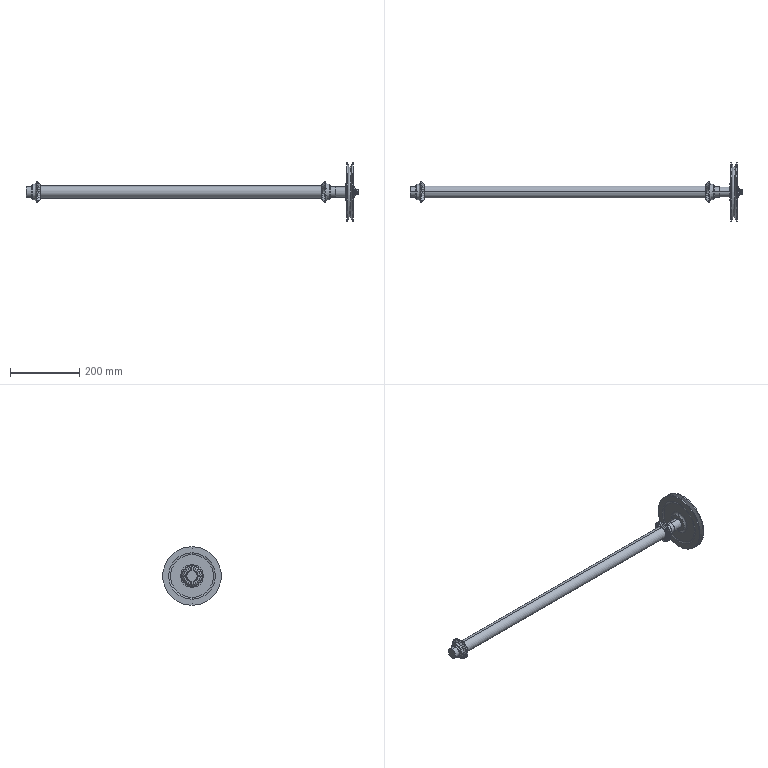Part | SolidWorks | 12 solids | 520 faces | box 961.9 x 169.7 x 169.7 mm | volume 1252859 mm3 | cone 154 | spline 144 | cylinder 120 | plane 74 | torus 28 | commonest cylinder face diameters 8 x35 31 x14 10 x10 28.4 x10 1.2 x8 30 x6